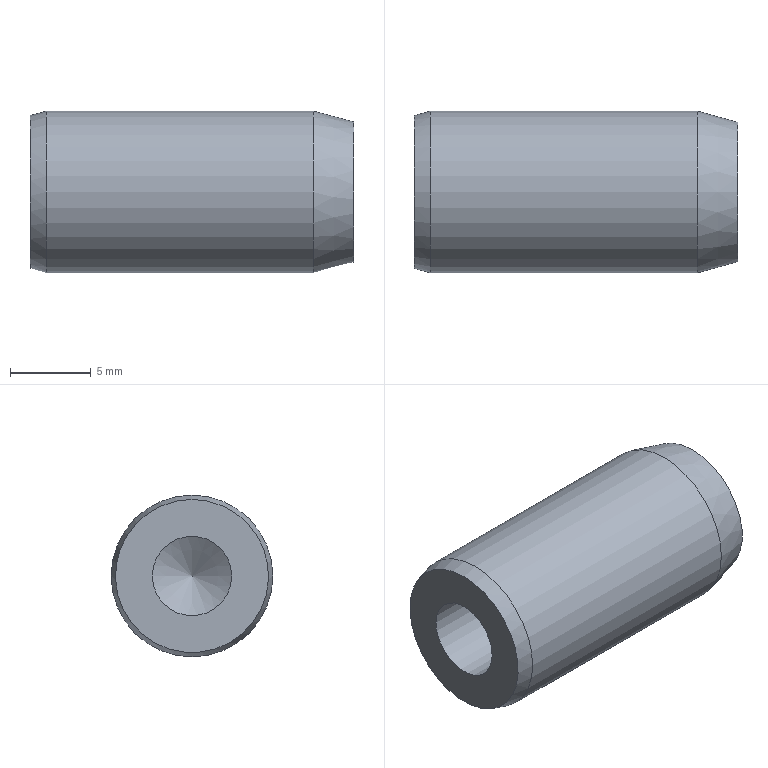Part | NX | features 5003_349_MSHT10-20(Default) 2 | 1 solid | 7 faces | box 20 x 10 x 10 mm | volume 1342 mm3 | cone 3 | plane 2 | cylinder 2 | commonest cylinder face diameters 4.917 x1 10 x1
STEP:
#1=CARTESIAN_POINT('',(386.89,-38.958,-149.25));
#2=VERTEX_POINT('',#1);
#3=CARTESIAN_POINT('',(386.89,-36.5,-149.25));
#4=DIRECTION('',(-1.,0.,0.));
#5=DIRECTION('',(0.,-1.,0.));
#6=AXIS2_PLACEMENT_3D('',#3,#4,#5);
#7=CIRCLE('',#6,2.458);
#8=EDGE_CURVE('',#2,#2,#7,.T.);
#9=ORIENTED_EDGE('',*,*,#8,.F.);
#10=EDGE_LOOP('',(#9));
#11=FACE_BOUND('',#10,.T.);
#12=CARTESIAN_POINT('',(386.89,-36.5,-144.518));
#13=VERTEX_POINT('',#12);
#14=CARTESIAN_POINT('',(386.89,-36.5,-149.25));
#15=DIRECTION('',(1.,0.,0.));
#16=DIRECTION('',(0.,0.,1.));
#17=AXIS2_PLACEMENT_3D('',#14,#15,#16);
#18=CIRCLE('',#17,4.732);
#19=EDGE_CURVE('',#13,#13,#18,.T.);
#20=ORIENTED_EDGE('',*,*,#19,.F.);
#21=EDGE_LOOP('',(#20));
#22=FACE_BOUND('',#21,.T.);
#23=CARTESIAN_POINT('',(386.89,-36.5,-149.25));
#24=DIRECTION('',(-1.,0.,0.));
#25=DIRECTION('',(0.,0.,-1.));
#26=AXIS2_PLACEMENT_3D('',#23,#24,#25);
#27=PLANE('',#26);
#28=ADVANCED_FACE('',(#11,#22),#27,.T.);
#29=ORIENTED_EDGE('',*,*,#19,.T.);
#30=EDGE_LOOP('',(#29));
#31=FACE_BOUND('',#30,.T.);
#32=CARTESIAN_POINT('',(387.89,-36.5,-144.25));
#33=VERTEX_POINT('',#32);
#34=CARTESIAN_POINT('',(387.89,-36.5,-149.25));
#35=DIRECTION('',(1.,0.,0.));
#36=DIRECTION('',(0.,0.,1.));
#37=AXIS2_PLACEMENT_3D('',#34,#35,#36);
#38=CIRCLE('',#37,5.);
#39=EDGE_CURVE('',#33,#33,#38,.T.);
#40=ORIENTED_EDGE('',*,*,#39,.F.);
#41=EDGE_LOOP('',(#40));
#42=FACE_BOUND('',#41,.T.);
#43=CARTESIAN_POINT('',(387.89,-36.5,-149.25));
#44=DIRECTION('',(1.,0.,0.));
#45=DIRECTION('',(0.,0.,1.));
#46=AXIS2_PLACEMENT_3D('',#43,#44,#45);
#47=CONICAL_SURFACE('',#46,5.,0.2618);
#48=ADVANCED_FACE('',(#31,#42),#47,.T.);
#49=ORIENTED_EDGE('',*,*,#39,.T.);
#50=EDGE_LOOP('',(#49));
#51=FACE_BOUND('',#50,.T.);
#52=CARTESIAN_POINT('',(404.39,-36.5,-144.25));
#53=VERTEX_POINT('',#52);
#54=CARTESIAN_POINT('',(404.39,-36.5,-149.25));
#55=DIRECTION('',(1.,0.,0.));
#56=DIRECTION('',(0.,0.,1.));
#57=AXIS2_PLACEMENT_3D('',#54,#55,#56);
#58=CIRCLE('',#57,5.);
#59=EDGE_CURVE('',#53,#53,#58,.T.);
#60=ORIENTED_EDGE('',*,*,#59,.F.);
#61=EDGE_LOOP('',(#60));
#62=FACE_BOUND('',#61,.T.);
#63=CARTESIAN_POINT('',(406.89,-36.5,-149.25));
#64=DIRECTION('',(1.,0.,0.));
#65=DIRECTION('',(0.,0.,1.));
#66=AXIS2_PLACEMENT_3D('',#63,#64,#65);
#67=CYLINDRICAL_SURFACE('',#66,5.);
#68=ADVANCED_FACE('',(#51,#62),#67,.T.);
#69=ORIENTED_EDGE('',*,*,#59,.T.);
#70=EDGE_LOOP('',(#69));
#71=FACE_BOUND('',#70,.T.);
#72=CARTESIAN_POINT('',(406.89,-36.5,-144.92));
#73=VERTEX_POINT('',#72);
#74=CARTESIAN_POINT('',(406.89,-36.5,-149.25));
#75=DIRECTION('',(1.,0.,0.));
#76=DIRECTION('',(0.,0.,1.));
#77=AXIS2_PLACEMENT_3D('',#74,#75,#76);
#78=CIRCLE('',#77,4.33);
#79=EDGE_CURVE('',#73,#73,#78,.T.);
#80=ORIENTED_EDGE('',*,*,#79,.F.);
#81=EDGE_LOOP('',(#80));
#82=FACE_BOUND('',#81,.T.);
#83=CARTESIAN_POINT('',(406.89,-36.5,-149.25));
#84=DIRECTION('',(-1.,0.,0.));
#85=DIRECTION('',(0.,0.,-1.));
#86=AXIS2_PLACEMENT_3D('',#83,#84,#85);
#87=CONICAL_SURFACE('',#86,4.33,0.2618);
#88=ADVANCED_FACE('',(#71,#82),#87,.T.);
#89=ORIENTED_EDGE('',*,*,#79,.T.);
#90=EDGE_LOOP('',(#89));
#91=FACE_BOUND('',#90,.T.);
#92=CARTESIAN_POINT('',(406.89,-36.5,-149.25));
#93=DIRECTION('',(1.,0.,0.));
#94=DIRECTION('',(0.,0.,1.));
#95=AXIS2_PLACEMENT_3D('',#92,#93,#94);
#96=PLANE('',#95);
#97=ADVANCED_FACE('',(#91),#96,.T.);
#98=CARTESIAN_POINT('',(398.368,-36.5,-149.25));
#99=VERTEX_POINT('',#98);
#100=VERTEX_LOOP('',#99);
#101=FACE_BOUND('',#100,.T.);
#102=CARTESIAN_POINT('',(396.89,-38.958,-149.25));
#103=VERTEX_POINT('',#102);
#104=CARTESIAN_POINT('',(396.89,-36.5,-149.25));
#105=DIRECTION('',(-1.,0.,0.));
#106=DIRECTION('',(0.,-1.,0.));
#107=AXIS2_PLACEMENT_3D('',#104,#105,#106);
#108=CIRCLE('',#107,2.458);
#109=EDGE_CURVE('',#103,#103,#108,.T.);
#110=ORIENTED_EDGE('',*,*,#109,.T.);
#111=EDGE_LOOP('',(#110));
#112=FACE_BOUND('',#111,.T.);
#113=CARTESIAN_POINT('',(396.89,-36.5,-149.25));
#114=DIRECTION('',(-1.,0.,0.));
#115=DIRECTION('',(0.,-1.,0.));
#116=AXIS2_PLACEMENT_3D('',#113,#114,#115);
#117=CONICAL_SURFACE('',#116,2.458,1.03);
#118=ADVANCED_FACE('',(#101,#112),#117,.F.);
#119=ORIENTED_EDGE('',*,*,#109,.F.);
#120=EDGE_LOOP('',(#119));
#121=FACE_BOUND('',#120,.T.);
#122=ORIENTED_EDGE('',*,*,#8,.T.);
#123=EDGE_LOOP('',(#122));
#124=FACE_BOUND('',#123,.T.);
#125=CARTESIAN_POINT('',(386.89,-36.5,-149.25));
#126=DIRECTION('',(-1.,0.,0.));
#127=DIRECTION('',(0.,-1.,0.));
#128=AXIS2_PLACEMENT_3D('',#125,#126,#127);
#129=CYLINDRICAL_SURFACE('',#128,2.458);
#130=ADVANCED_FACE('',(#121,#124),#129,.F.);
#131=CLOSED_SHELL('',(#28,#48,#68,#88,#97,#118,#130));
#132=MANIFOLD_SOLID_BREP('',#131);
#133=(LENGTH_UNIT()NAMED_UNIT(*)SI_UNIT(.MILLI.,.METRE.));
#134=UNCERTAINTY_MEASURE_WITH_UNIT(LENGTH_MEASURE(0.00001),#133,'','');
#135=(NAMED_UNIT(*)PLANE_ANGLE_UNIT()SI_UNIT($,.RADIAN.));
#136=(NAMED_UNIT(*)SI_UNIT($,.STERADIAN.)SOLID_ANGLE_UNIT());
#137=(GEOMETRIC_REPRESENTATION_CONTEXT(3)GLOBAL_UNCERTAINTY_ASSIGNED_CONTEXT((#134))GLOBAL_UNIT_ASSIGNED_CONTEXT((#133,#135,#136))REPRESENTATION_CONTEXT('',''));
#138=ADVANCED_BREP_SHAPE_REPRESENTATION('',(#132),#137);